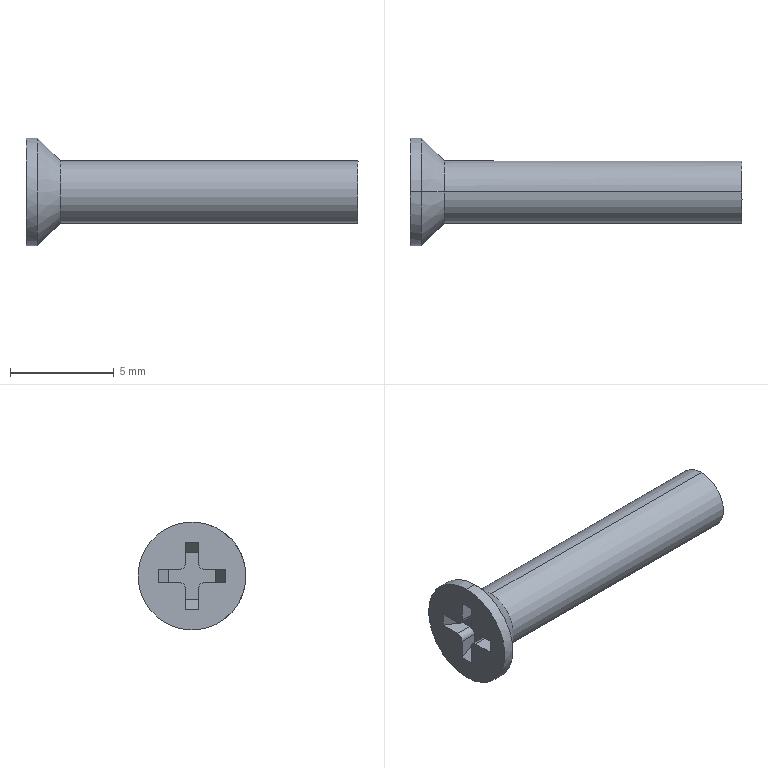Part | STEP file | PN_0006_Default<As Machined> | 1 solid | 25 faces | box 16 x 5.2 x 5.2 mm | volume 125.378 mm3 | plane 15 | cylinder 8 | cone 2 | commonest cylinder face diameters 0.6 x4 3 x2 5.2 x2
STEP:
#1=CARTESIAN_POINT('',(1.65,0.,-1.5));
#2=VERTEX_POINT('',#1);
#3=CARTESIAN_POINT('',(1.65,0.,1.5));
#4=VERTEX_POINT('',#3);
#5=CARTESIAN_POINT('',(1.65,0.,-1.5));
#6=CARTESIAN_POINT('',(1.65,0.4712,-1.5));
#7=CARTESIAN_POINT('',(1.65,0.9425,-1.315));
#8=CARTESIAN_POINT('',(1.65,1.315,-0.9425));
#9=CARTESIAN_POINT('',(1.65,1.685,0.));
#10=CARTESIAN_POINT('',(1.65,1.315,0.9425));
#11=CARTESIAN_POINT('',(1.65,0.9425,1.315));
#12=CARTESIAN_POINT('',(1.65,0.4712,1.5));
#13=CARTESIAN_POINT('',(1.65,0.,1.5));
#14=B_SPLINE_CURVE_WITH_KNOTS('',5,(#5,#6,#7,#8,#9,#10,#11,#12,#13),.UNSPECIFIED.,.F.,.U.,(6,3,6),(-2.356,0.,2.356),.UNSPECIFIED.);
#15=EDGE_CURVE('',#2,#4,#14,.T.);
#16=ORIENTED_EDGE('',*,*,#15,.T.);
#17=CARTESIAN_POINT('',(16.,0.,1.5));
#18=VERTEX_POINT('',#17);
#19=CARTESIAN_POINT('',(4.516,0.,1.5));
#20=DIRECTION('',(1.,0.,0.));
#21=VECTOR('',#20,1.);
#22=LINE('',#19,#21);
#23=EDGE_CURVE('',#4,#18,#22,.T.);
#24=ORIENTED_EDGE('',*,*,#23,.T.);
#25=CARTESIAN_POINT('',(16.,0.,-1.5));
#26=VERTEX_POINT('',#25);
#27=CARTESIAN_POINT('',(16.,0.,0.));
#28=DIRECTION('',(1.,0.,0.));
#29=AXIS2_PLACEMENT_3D('',#27,#28,$);
#30=CIRCLE('',#29,1.5);
#31=EDGE_CURVE('',#26,#18,#30,.T.);
#32=ORIENTED_EDGE('',*,*,#31,.F.);
#33=CARTESIAN_POINT('',(4.516,0.,-1.5));
#34=DIRECTION('',(1.,0.,0.));
#35=VECTOR('',#34,1.);
#36=LINE('',#33,#35);
#37=EDGE_CURVE('',#2,#26,#36,.T.);
#38=ORIENTED_EDGE('',*,*,#37,.F.);
#39=EDGE_LOOP('',(#16,#24,#32,#38));
#40=FACE_OUTER_BOUND('',#39,.T.);
#41=CARTESIAN_POINT('',(4.516,0.,0.));
#42=DIRECTION('',(1.,0.,0.));
#43=DIRECTION('',(0.,0.,-1.));
#44=AXIS2_PLACEMENT_3D('',#41,#42,#43);
#45=CYLINDRICAL_SURFACE('',#44,1.5);
#46=ADVANCED_FACE('',(#40),#45,.T.);
#47=ORIENTED_EDGE('',*,*,#15,.F.);
#48=CARTESIAN_POINT('',(0.55,0.,-2.6));
#49=VERTEX_POINT('',#48);
#50=CARTESIAN_POINT('',(-353550.991,0.,-353554.141));
#51=DIRECTION('',(-0.7071,0.,-0.7071));
#52=VECTOR('',#51,1.);
#53=LINE('',#50,#52);
#54=EDGE_CURVE('',#2,#49,#53,.T.);
#55=ORIENTED_EDGE('',*,*,#54,.T.);
#56=CARTESIAN_POINT('',(0.55,0.,2.6));
#57=VERTEX_POINT('',#56);
#58=CARTESIAN_POINT('',(0.55,0.,0.));
#59=DIRECTION('',(-1.,0.,0.));
#60=AXIS2_PLACEMENT_3D('',#58,#59,$);
#61=CIRCLE('',#60,2.6);
#62=EDGE_CURVE('',#49,#57,#61,.F.);
#63=ORIENTED_EDGE('',*,*,#62,.T.);
#64=CARTESIAN_POINT('',(-353550.991,0.,353554.141));
#65=DIRECTION('',(-0.7071,0.,0.7071));
#66=VECTOR('',#65,1.);
#67=LINE('',#64,#66);
#68=EDGE_CURVE('',#4,#57,#67,.T.);
#69=ORIENTED_EDGE('',*,*,#68,.F.);
#70=EDGE_LOOP('',(#47,#55,#63,#69));
#71=FACE_OUTER_BOUND('',#70,.T.);
#72=CARTESIAN_POINT('',(1.65,0.,0.));
#73=DIRECTION('',(-1.,0.,0.));
#74=DIRECTION('',(0.,0.,1.));
#75=AXIS2_PLACEMENT_3D('',#72,#73,#74);
#76=CONICAL_SURFACE('',#75,1.5,0.7854);
#77=ADVANCED_FACE('',(#71),#76,.T.);
#78=ORIENTED_EDGE('',*,*,#23,.F.);
#79=CARTESIAN_POINT('',(1.65,0.,1.5));
#80=CARTESIAN_POINT('',(1.65,-0.4712,1.5));
#81=CARTESIAN_POINT('',(1.65,-0.9425,1.315));
#82=CARTESIAN_POINT('',(1.65,-1.315,0.9425));
#83=CARTESIAN_POINT('',(1.65,-1.685,0.));
#84=CARTESIAN_POINT('',(1.65,-1.315,-0.9425));
#85=CARTESIAN_POINT('',(1.65,-0.9425,-1.315));
#86=CARTESIAN_POINT('',(1.65,-0.4712,-1.5));
#87=CARTESIAN_POINT('',(1.65,0.,-1.5));
#88=B_SPLINE_CURVE_WITH_KNOTS('',5,(#79,#80,#81,#82,#83,#84,#85,#86,#87),.UNSPECIFIED.,.F.,.U.,(6,3,6),(-2.356,0.,2.356),.UNSPECIFIED.);
#89=EDGE_CURVE('',#4,#2,#88,.T.);
#90=ORIENTED_EDGE('',*,*,#89,.T.);
#91=ORIENTED_EDGE('',*,*,#37,.T.);
#92=CARTESIAN_POINT('',(16.,0.,1.5));
#93=CARTESIAN_POINT('',(16.,-0.4712,1.5));
#94=CARTESIAN_POINT('',(16.,-0.9425,1.315));
#95=CARTESIAN_POINT('',(16.,-1.315,0.9425));
#96=CARTESIAN_POINT('',(16.,-1.685,0.));
#97=CARTESIAN_POINT('',(16.,-1.315,-0.9425));
#98=CARTESIAN_POINT('',(16.,-0.9425,-1.315));
#99=CARTESIAN_POINT('',(16.,-0.4712,-1.5));
#100=CARTESIAN_POINT('',(16.,0.,-1.5));
#101=B_SPLINE_CURVE_WITH_KNOTS('',5,(#92,#93,#94,#95,#96,#97,#98,#99,#100),.UNSPECIFIED.,.F.,.U.,(6,3,6),(-2.356,0.,2.356),.UNSPECIFIED.);
#102=EDGE_CURVE('',#18,#26,#101,.T.);
#103=ORIENTED_EDGE('',*,*,#102,.F.);
#104=EDGE_LOOP('',(#78,#90,#91,#103));
#105=FACE_OUTER_BOUND('',#104,.T.);
#106=CARTESIAN_POINT('',(4.516,0.,0.));
#107=DIRECTION('',(1.,0.,0.));
#108=DIRECTION('',(0.,0.,1.));
#109=AXIS2_PLACEMENT_3D('',#106,#107,#108);
#110=CYLINDRICAL_SURFACE('',#109,1.5);
#111=ADVANCED_FACE('',(#105),#110,.T.);
#112=ORIENTED_EDGE('',*,*,#31,.T.);
#113=ORIENTED_EDGE('',*,*,#102,.T.);
#114=EDGE_LOOP('',(#112,#113));
#115=FACE_OUTER_BOUND('',#114,.T.);
#116=CARTESIAN_POINT('',(16.,1.5,0.));
#117=DIRECTION('',(1.,0.,0.));
#118=DIRECTION('',(0.,0.,-1.));
#119=AXIS2_PLACEMENT_3D('',#116,#117,#118);
#120=PLANE('',#119);
#121=ADVANCED_FACE('',(#115),#120,.T.);
#122=ORIENTED_EDGE('',*,*,#54,.F.);
#123=ORIENTED_EDGE('',*,*,#89,.F.);
#124=ORIENTED_EDGE('',*,*,#68,.T.);
#125=CARTESIAN_POINT('',(0.55,0.,0.));
#126=DIRECTION('',(-1.,0.,0.));
#127=AXIS2_PLACEMENT_3D('',#125,#126,$);
#128=CIRCLE('',#127,2.6);
#129=EDGE_CURVE('',#57,#49,#128,.F.);
#130=ORIENTED_EDGE('',*,*,#129,.T.);
#131=EDGE_LOOP('',(#122,#123,#124,#130));
#132=FACE_OUTER_BOUND('',#131,.T.);
#133=CARTESIAN_POINT('',(1.65,0.,0.));
#134=DIRECTION('',(-1.,0.,0.));
#135=DIRECTION('',(0.,0.,-1.));
#136=AXIS2_PLACEMENT_3D('',#133,#134,#135);
#137=CONICAL_SURFACE('',#136,1.5,0.7854);
#138=ADVANCED_FACE('',(#132),#137,.T.);
#139=CARTESIAN_POINT('',(0.,0.,-2.6));
#140=VERTEX_POINT('',#139);
#141=CARTESIAN_POINT('',(0.,0.,2.6));
#142=VERTEX_POINT('',#141);
#143=CARTESIAN_POINT('',(0.,0.,0.));
#144=DIRECTION('',(1.,0.,0.));
#145=AXIS2_PLACEMENT_3D('',#143,#144,$);
#146=CIRCLE('',#145,2.6);
#147=EDGE_CURVE('',#140,#142,#146,.T.);
#148=ORIENTED_EDGE('',*,*,#147,.T.);
#149=CARTESIAN_POINT('',(4.516,0.,2.6));
#150=DIRECTION('',(1.,0.,0.));
#151=VECTOR('',#150,1.);
#152=LINE('',#149,#151);
#153=EDGE_CURVE('',#142,#57,#152,.T.);
#154=ORIENTED_EDGE('',*,*,#153,.T.);
#155=ORIENTED_EDGE('',*,*,#62,.F.);
#156=CARTESIAN_POINT('',(4.516,0.,-2.6));
#157=DIRECTION('',(1.,0.,0.));
#158=VECTOR('',#157,1.);
#159=LINE('',#156,#158);
#160=EDGE_CURVE('',#140,#49,#159,.T.);
#161=ORIENTED_EDGE('',*,*,#160,.F.);
#162=EDGE_LOOP('',(#148,#154,#155,#161));
#163=FACE_OUTER_BOUND('',#162,.T.);
#164=CARTESIAN_POINT('',(4.516,0.,0.));
#165=DIRECTION('',(1.,0.,0.));
#166=DIRECTION('',(0.,0.,-1.));
#167=AXIS2_PLACEMENT_3D('',#164,#165,#166);
#168=CYLINDRICAL_SURFACE('',#167,2.6);
#169=ADVANCED_FACE('',(#163),#168,.T.);
#170=ORIENTED_EDGE('',*,*,#153,.F.);
#171=CARTESIAN_POINT('',(0.,0.,2.6));
#172=CARTESIAN_POINT('',(0.,-0.8168,2.6));
#173=CARTESIAN_POINT('',(0.,-1.634,2.279));
#174=CARTESIAN_POINT('',(0.,-2.279,1.634));
#175=CARTESIAN_POINT('',(0.,-2.921,0.));
#176=CARTESIAN_POINT('',(0.,-2.279,-1.634));
#177=CARTESIAN_POINT('',(0.,-1.634,-2.279));
#178=CARTESIAN_POINT('',(0.,-0.8168,-2.6));
#179=CARTESIAN_POINT('',(0.,0.,-2.6));
#180=B_SPLINE_CURVE_WITH_KNOTS('',5,(#171,#172,#173,#174,#175,#176,#177,#178,#179),.UNSPECIFIED.,.F.,.U.,(6,3,6),(-4.084,0.,4.084),.UNSPECIFIED.);
#181=EDGE_CURVE('',#142,#140,#180,.T.);
#182=ORIENTED_EDGE('',*,*,#181,.T.);
#183=ORIENTED_EDGE('',*,*,#160,.T.);
#184=ORIENTED_EDGE('',*,*,#129,.F.);
#185=EDGE_LOOP('',(#170,#182,#183,#184));
#186=FACE_OUTER_BOUND('',#185,.T.);
#187=CARTESIAN_POINT('',(4.516,0.,0.));
#188=DIRECTION('',(1.,0.,0.));
#189=DIRECTION('',(0.,0.,1.));
#190=AXIS2_PLACEMENT_3D('',#187,#188,#189);
#191=CYLINDRICAL_SURFACE('',#190,2.6);
#192=ADVANCED_FACE('',(#186),#191,.T.);
#193=ORIENTED_EDGE('',*,*,#147,.F.);
#194=ORIENTED_EDGE('',*,*,#181,.F.);
#195=EDGE_LOOP('',(#193,#194));
#196=FACE_OUTER_BOUND('',#195,.T.);
#197=CARTESIAN_POINT('',(0.,-1.6,-0.32));
#198=VERTEX_POINT('',#197);
#199=CARTESIAN_POINT('',(0.,-0.62,-0.32));
#200=VERTEX_POINT('',#199);
#201=CARTESIAN_POINT('',(0.,-1.11,-0.32));
#202=DIRECTION('',(0.,1.,0.));
#203=VECTOR('',#202,1.);
#204=LINE('',#201,#203);
#205=EDGE_CURVE('',#198,#200,#204,.T.);
#206=ORIENTED_EDGE('',*,*,#205,.T.);
#207=CARTESIAN_POINT('',(0.,-0.32,-0.62));
#208=VERTEX_POINT('',#207);
#209=CARTESIAN_POINT('',(0.,-0.62,-0.62));
#210=DIRECTION('',(-1.,0.,0.));
#211=AXIS2_PLACEMENT_3D('',#209,#210,$);
#212=CIRCLE('',#211,0.3);
#213=EDGE_CURVE('',#200,#208,#212,.T.);
#214=ORIENTED_EDGE('',*,*,#213,.T.);
#215=CARTESIAN_POINT('',(0.,-0.32,-1.6));
#216=VERTEX_POINT('',#215);
#217=CARTESIAN_POINT('',(0.,-0.32,-1.11));
#218=DIRECTION('',(0.,0.,-1.));
#219=VECTOR('',#218,1.);
#220=LINE('',#217,#219);
#221=EDGE_CURVE('',#208,#216,#220,.T.);
#222=ORIENTED_EDGE('',*,*,#221,.T.);
#223=CARTESIAN_POINT('',(0.,0.32,-1.6));
#224=VERTEX_POINT('',#223);
#225=CARTESIAN_POINT('',(0.,0.,-1.6));
#226=DIRECTION('',(0.,1.,0.));
#227=VECTOR('',#226,1.);
#228=LINE('',#225,#227);
#229=EDGE_CURVE('',#216,#224,#228,.T.);
#230=ORIENTED_EDGE('',*,*,#229,.T.);
#231=CARTESIAN_POINT('',(0.,0.32,-0.62));
#232=VERTEX_POINT('',#231);
#233=CARTESIAN_POINT('',(0.,0.32,-1.11));
#234=DIRECTION('',(0.,0.,1.));
#235=VECTOR('',#234,1.);
#236=LINE('',#233,#235);
#237=EDGE_CURVE('',#224,#232,#236,.T.);
#238=ORIENTED_EDGE('',*,*,#237,.T.);
#239=CARTESIAN_POINT('',(0.,0.62,-0.32));
#240=VERTEX_POINT('',#239);
#241=CARTESIAN_POINT('',(0.,0.62,-0.62));
#242=DIRECTION('',(-1.,0.,0.));
#243=AXIS2_PLACEMENT_3D('',#241,#242,$);
#244=CIRCLE('',#243,0.3);
#245=EDGE_CURVE('',#232,#240,#244,.T.);
#246=ORIENTED_EDGE('',*,*,#245,.T.);
#247=CARTESIAN_POINT('',(0.,1.6,-0.32));
#248=VERTEX_POINT('',#247);
#249=CARTESIAN_POINT('',(0.,1.11,-0.32));
#250=DIRECTION('',(0.,1.,0.));
#251=VECTOR('',#250,1.);
#252=LINE('',#249,#251);
#253=EDGE_CURVE('',#240,#248,#252,.T.);
#254=ORIENTED_EDGE('',*,*,#253,.T.);
#255=CARTESIAN_POINT('',(0.,1.6,0.32));
#256=VERTEX_POINT('',#255);
#257=CARTESIAN_POINT('',(0.,1.6,0.));
#258=DIRECTION('',(0.,0.,1.));
#259=VECTOR('',#258,1.);
#260=LINE('',#257,#259);
#261=EDGE_CURVE('',#248,#256,#260,.T.);
#262=ORIENTED_EDGE('',*,*,#261,.T.);
#263=CARTESIAN_POINT('',(0.,0.62,0.32));
#264=VERTEX_POINT('',#263);
#265=CARTESIAN_POINT('',(0.,1.11,0.32));
#266=DIRECTION('',(0.,-1.,0.));
#267=VECTOR('',#266,1.);
#268=LINE('',#265,#267);
#269=EDGE_CURVE('',#256,#264,#268,.T.);
#270=ORIENTED_EDGE('',*,*,#269,.T.);
#271=CARTESIAN_POINT('',(0.,0.32,0.62));
#272=VERTEX_POINT('',#271);
#273=CARTESIAN_POINT('',(0.,0.62,0.62));
#274=DIRECTION('',(-1.,0.,0.));
#275=AXIS2_PLACEMENT_3D('',#273,#274,$);
#276=CIRCLE('',#275,0.3);
#277=EDGE_CURVE('',#264,#272,#276,.T.);
#278=ORIENTED_EDGE('',*,*,#277,.T.);
#279=CARTESIAN_POINT('',(0.,0.32,1.6));
#280=VERTEX_POINT('',#279);
#281=CARTESIAN_POINT('',(0.,0.32,1.11));
#282=DIRECTION('',(0.,0.,1.));
#283=VECTOR('',#282,1.);
#284=LINE('',#281,#283);
#285=EDGE_CURVE('',#272,#280,#284,.T.);
#286=ORIENTED_EDGE('',*,*,#285,.T.);
#287=CARTESIAN_POINT('',(0.,-0.32,1.6));
#288=VERTEX_POINT('',#287);
#289=CARTESIAN_POINT('',(0.,0.,1.6));
#290=DIRECTION('',(0.,-1.,0.));
#291=VECTOR('',#290,1.);
#292=LINE('',#289,#291);
#293=EDGE_CURVE('',#280,#288,#292,.T.);
#294=ORIENTED_EDGE('',*,*,#293,.T.);
#295=CARTESIAN_POINT('',(0.,-0.32,0.62));
#296=VERTEX_POINT('',#295);
#297=CARTESIAN_POINT('',(0.,-0.32,1.11));
#298=DIRECTION('',(0.,0.,-1.));
#299=VECTOR('',#298,1.);
#300=LINE('',#297,#299);
#301=EDGE_CURVE('',#288,#296,#300,.T.);
#302=ORIENTED_EDGE('',*,*,#301,.T.);
#303=CARTESIAN_POINT('',(0.,-0.62,0.32));
#304=VERTEX_POINT('',#303);
#305=CARTESIAN_POINT('',(0.,-0.62,0.62));
#306=DIRECTION('',(-1.,0.,0.));
#307=AXIS2_PLACEMENT_3D('',#305,#306,$);
#308=CIRCLE('',#307,0.3);
#309=EDGE_CURVE('',#296,#304,#308,.T.);
#310=ORIENTED_EDGE('',*,*,#309,.T.);
#311=CARTESIAN_POINT('',(0.,-1.6,0.32));
#312=VERTEX_POINT('',#311);
#313=CARTESIAN_POINT('',(0.,-1.11,0.32));
#314=DIRECTION('',(0.,-1.,0.));
#315=VECTOR('',#314,1.);
#316=LINE('',#313,#315);
#317=EDGE_CURVE('',#304,#312,#316,.T.);
#318=ORIENTED_EDGE('',*,*,#317,.T.);
#319=CARTESIAN_POINT('',(0.,-1.6,0.));
#320=DIRECTION('',(0.,0.,-1.));
#321=VECTOR('',#320,1.);
#322=LINE('',#319,#321);
#323=EDGE_CURVE('',#312,#198,#322,.T.);
#324=ORIENTED_EDGE('',*,*,#323,.T.);
#325=EDGE_LOOP('',(#206,#214,#222,#230,#238,#246,#254,#262,#270,#278,#286,#294,#302,#310,#318,#324));
#326=FACE_BOUND('',#325,.T.);
#327=CARTESIAN_POINT('',(0.,2.6,0.));
#328=DIRECTION('',(-1.,0.,0.));
#329=DIRECTION('',(0.,0.,1.));
#330=AXIS2_PLACEMENT_3D('',#327,#328,#329);
#331=PLANE('',#330);
#332=ADVANCED_FACE('',(#196,#326),#331,.T.);
#333=CARTESIAN_POINT('',(0.825,-1.124,-0.32));
#334=VERTEX_POINT('',#333);
#335=CARTESIAN_POINT('',(0.825,-0.62,-0.32));
#336=VERTEX_POINT('',#335);
#337=CARTESIAN_POINT('',(0.825,-0.8718,-0.32));
#338=DIRECTION('',(0.,1.,0.));
#339=VECTOR('',#338,1.);
#340=LINE('',#337,#339);
#341=EDGE_CURVE('',#334,#336,#340,.T.);
#342=ORIENTED_EDGE('',*,*,#341,.T.);
#343=CARTESIAN_POINT('',(0.4125,-0.62,-0.32));
#344=DIRECTION('',(-1.,0.,0.));
#345=VECTOR('',#344,1.);
#346=LINE('',#343,#345);
#347=EDGE_CURVE('',#336,#200,#346,.T.);
#348=ORIENTED_EDGE('',*,*,#347,.T.);
#349=ORIENTED_EDGE('',*,*,#205,.F.);
#350=CARTESIAN_POINT('',(0.4125,-1.362,-0.32));
#351=DIRECTION('',(-0.866,-0.5,0.));
#352=VECTOR('',#351,1.);
#353=LINE('',#350,#352);
#354=EDGE_CURVE('',#334,#198,#353,.T.);
#355=ORIENTED_EDGE('',*,*,#354,.F.);
#356=EDGE_LOOP('',(#342,#348,#349,#355));
#357=FACE_OUTER_BOUND('',#356,.T.);
#358=CARTESIAN_POINT('',(0.825,-0.32,-0.32));
#359=DIRECTION('',(0.,0.,1.));
#360=DIRECTION('',(1.,0.,0.));
#361=AXIS2_PLACEMENT_3D('',#358,#359,#360);
#362=PLANE('',#361);
#363=ADVANCED_FACE('',(#357),#362,.T.);
#364=CARTESIAN_POINT('',(0.825,-0.32,-0.62));
#365=VERTEX_POINT('',#364);
#366=CARTESIAN_POINT('',(0.825,-0.62,-0.62));
#367=DIRECTION('',(-1.,0.,0.));
#368=AXIS2_PLACEMENT_3D('',#366,#367,$);
#369=CIRCLE('',#368,0.3);
#370=EDGE_CURVE('',#365,#336,#369,.F.);
#371=ORIENTED_EDGE('',*,*,#370,.F.);
#372=CARTESIAN_POINT('',(0.825,-0.32,-0.62));
#373=DIRECTION('',(-1.,0.,0.));
#374=VECTOR('',#373,1.);
#375=LINE('',#372,#374);
#376=EDGE_CURVE('',#208,#365,#375,.F.);
#377=ORIENTED_EDGE('',*,*,#376,.F.);
#378=ORIENTED_EDGE('',*,*,#213,.F.);
#379=ORIENTED_EDGE('',*,*,#347,.F.);
#380=EDGE_LOOP('',(#371,#377,#378,#379));
#381=FACE_OUTER_BOUND('',#380,.T.);
#382=CARTESIAN_POINT('',(0.825,-0.62,-0.62));
#383=DIRECTION('',(-1.,0.,0.));
#384=DIRECTION('',(0.,0.,1.));
#385=AXIS2_PLACEMENT_3D('',#382,#383,#384);
#386=CYLINDRICAL_SURFACE('',#385,0.3);
#387=ADVANCED_FACE('',(#381),#386,.T.);
#388=ORIENTED_EDGE('',*,*,#221,.F.);
#389=ORIENTED_EDGE('',*,*,#376,.T.);
#390=CARTESIAN_POINT('',(0.825,-0.32,-1.124));
#391=VERTEX_POINT('',#390);
#392=CARTESIAN_POINT('',(0.825,-0.32,-0.8718));
#393=DIRECTION('',(0.,0.,-1.));
#394=VECTOR('',#393,1.);
#395=LINE('',#392,#394);
#396=EDGE_CURVE('',#365,#391,#395,.T.);
#397=ORIENTED_EDGE('',*,*,#396,.T.);
#398=CARTESIAN_POINT('',(0.4125,-0.32,-1.362));
#399=DIRECTION('',(-0.866,0.,-0.5));
#400=VECTOR('',#399,1.);
#401=LINE('',#398,#400);
#402=EDGE_CURVE('',#391,#216,#401,.T.);
#403=ORIENTED_EDGE('',*,*,#402,.T.);
#404=EDGE_LOOP('',(#388,#389,#397,#403));
#405=FACE_OUTER_BOUND('',#404,.T.);
#406=CARTESIAN_POINT('',(0.825,-0.32,-0.32));
#407=DIRECTION('',(0.,1.,0.));
#408=DIRECTION('',(0.,0.,1.));
#409=AXIS2_PLACEMENT_3D('',#406,#407,#408);
#410=PLANE('',#409);
#411=ADVANCED_FACE('',(#405),#410,.T.);
#412=ORIENTED_EDGE('',*,*,#229,.F.);
#413=ORIENTED_EDGE('',*,*,#402,.F.);
#414=CARTESIAN_POINT('',(0.825,0.32,-1.124));
#415=VERTEX_POINT('',#414);
#416=CARTESIAN_POINT('',(0.825,0.,-1.124));
#417=DIRECTION('',(0.,1.,0.));
#418=VECTOR('',#417,1.);
#419=LINE('',#416,#418);
#420=EDGE_CURVE('',#391,#415,#419,.T.);
#421=ORIENTED_EDGE('',*,*,#420,.T.);
#422=CARTESIAN_POINT('',(0.4125,0.32,-1.362));
#423=DIRECTION('',(-0.866,0.,-0.5));
#424=VECTOR('',#423,1.);
#425=LINE('',#422,#424);
#426=EDGE_CURVE('',#415,#224,#425,.T.);
#427=ORIENTED_EDGE('',*,*,#426,.T.);
#428=EDGE_LOOP('',(#412,#413,#421,#427));
#429=FACE_OUTER_BOUND('',#428,.T.);
#430=CARTESIAN_POINT('',(0.,0.32,-1.6));
#431=DIRECTION('',(-0.5,0.,0.866));
#432=DIRECTION('',(0.866,0.,0.5));
#433=AXIS2_PLACEMENT_3D('',#430,#431,#432);
#434=PLANE('',#433);
#435=ADVANCED_FACE('',(#429),#434,.T.);
#436=CARTESIAN_POINT('',(0.825,0.32,-0.62));
#437=VERTEX_POINT('',#436);
#438=CARTESIAN_POINT('',(0.825,0.32,-0.8718));
#439=DIRECTION('',(0.,0.,1.));
#440=VECTOR('',#439,1.);
#441=LINE('',#438,#440);
#442=EDGE_CURVE('',#415,#437,#441,.T.);
#443=ORIENTED_EDGE('',*,*,#442,.T.);
#444=CARTESIAN_POINT('',(0.4125,0.32,-0.62));
#445=DIRECTION('',(-1.,0.,0.));
#446=VECTOR('',#445,1.);
#447=LINE('',#444,#446);
#448=EDGE_CURVE('',#437,#232,#447,.T.);
#449=ORIENTED_EDGE('',*,*,#448,.T.);
#450=ORIENTED_EDGE('',*,*,#237,.F.);
#451=ORIENTED_EDGE('',*,*,#426,.F.);
#452=EDGE_LOOP('',(#443,#449,#450,#451));
#453=FACE_OUTER_BOUND('',#452,.T.);
#454=CARTESIAN_POINT('',(0.825,0.32,-0.32));
#455=DIRECTION('',(0.,-1.,0.));
#456=DIRECTION('',(0.,0.,-1.));
#457=AXIS2_PLACEMENT_3D('',#454,#455,#456);
#458=PLANE('',#457);
#459=ADVANCED_FACE('',(#453),#458,.T.);
#460=CARTESIAN_POINT('',(0.825,0.62,-0.32));
#461=VERTEX_POINT('',#460);
#462=CARTESIAN_POINT('',(0.825,0.62,-0.62));
#463=DIRECTION('',(-1.,0.,0.));
#464=AXIS2_PLACEMENT_3D('',#462,#463,$);
#465=CIRCLE('',#464,0.3);
#466=EDGE_CURVE('',#461,#437,#465,.F.);
#467=ORIENTED_EDGE('',*,*,#466,.F.);
#468=CARTESIAN_POINT('',(0.825,0.62,-0.32));
#469=DIRECTION('',(-1.,0.,0.));
#470=VECTOR('',#469,1.);
#471=LINE('',#468,#470);
#472=EDGE_CURVE('',#240,#461,#471,.F.);
#473=ORIENTED_EDGE('',*,*,#472,.F.);
#474=ORIENTED_EDGE('',*,*,#245,.F.);
#475=ORIENTED_EDGE('',*,*,#448,.F.);
#476=EDGE_LOOP('',(#467,#473,#474,#475));
#477=FACE_OUTER_BOUND('',#476,.T.);
#478=CARTESIAN_POINT('',(0.825,0.62,-0.62));
#479=DIRECTION('',(-1.,0.,0.));
#480=DIRECTION('',(0.,0.,-1.));
#481=AXIS2_PLACEMENT_3D('',#478,#479,#480);
#482=CYLINDRICAL_SURFACE('',#481,0.3);
#483=ADVANCED_FACE('',(#477),#482,.T.);
#484=ORIENTED_EDGE('',*,*,#253,.F.);
#485=ORIENTED_EDGE('',*,*,#472,.T.);
#486=CARTESIAN_POINT('',(0.825,1.124,-0.32));
#487=VERTEX_POINT('',#486);
#488=CARTESIAN_POINT('',(0.825,0.8718,-0.32));
#489=DIRECTION('',(0.,1.,0.));
#490=VECTOR('',#489,1.);
#491=LINE('',#488,#490);
#492=EDGE_CURVE('',#461,#487,#491,.T.);
#493=ORIENTED_EDGE('',*,*,#492,.T.);
#494=CARTESIAN_POINT('',(0.4125,1.362,-0.32));
#495=DIRECTION('',(-0.866,0.5,0.));
#496=VECTOR('',#495,1.);
#497=LINE('',#494,#496);
#498=EDGE_CURVE('',#487,#248,#497,.T.);
#499=ORIENTED_EDGE('',*,*,#498,.T.);
#500=EDGE_LOOP('',(#484,#485,#493,#499));
#501=FACE_OUTER_BOUND('',#500,.T.);
#502=CARTESIAN_POINT('',(0.825,0.32,-0.32));
#503=DIRECTION('',(0.,0.,1.));
#504=DIRECTION('',(1.,0.,0.));
#505=AXIS2_PLACEMENT_3D('',#502,#503,#504);
#506=PLANE('',#505);
#507=ADVANCED_FACE('',(#501),#506,.T.);
#508=ORIENTED_EDGE('',*,*,#261,.F.);
#509=ORIENTED_EDGE('',*,*,#498,.F.);
#510=CARTESIAN_POINT('',(0.825,1.124,0.32));
#511=VERTEX_POINT('',#510);
#512=CARTESIAN_POINT('',(0.825,1.124,0.));
#513=DIRECTION('',(0.,0.,1.));
#514=VECTOR('',#513,1.);
#515=LINE('',#512,#514);
#516=EDGE_CURVE('',#487,#511,#515,.T.);
#517=ORIENTED_EDGE('',*,*,#516,.T.);
#518=CARTESIAN_POINT('',(0.4125,1.362,0.32));
#519=DIRECTION('',(-0.866,0.5,0.));
#520=VECTOR('',#519,1.);
#521=LINE('',#518,#520);
#522=EDGE_CURVE('',#511,#256,#521,.T.);
#523=ORIENTED_EDGE('',*,*,#522,.T.);
#524=EDGE_LOOP('',(#508,#509,#517,#523));
#525=FACE_OUTER_BOUND('',#524,.T.);
#526=CARTESIAN_POINT('',(0.,1.6,-0.32));
#527=DIRECTION('',(-0.5,-0.866,0.));
#528=DIRECTION('',(0.866,-0.5,0.));
#529=AXIS2_PLACEMENT_3D('',#526,#527,#528);
#530=PLANE('',#529);
#531=ADVANCED_FACE('',(#525),#530,.T.);
#532=CARTESIAN_POINT('',(0.825,0.62,0.32));
#533=VERTEX_POINT('',#532);
#534=CARTESIAN_POINT('',(0.825,0.8718,0.32));
#535=DIRECTION('',(0.,-1.,0.));
#536=VECTOR('',#535,1.);
#537=LINE('',#534,#536);
#538=EDGE_CURVE('',#511,#533,#537,.T.);
#539=ORIENTED_EDGE('',*,*,#538,.T.);
#540=CARTESIAN_POINT('',(0.4125,0.62,0.32));
#541=DIRECTION('',(-1.,0.,0.));
#542=VECTOR('',#541,1.);
#543=LINE('',#540,#542);
#544=EDGE_CURVE('',#533,#264,#543,.T.);
#545=ORIENTED_EDGE('',*,*,#544,.T.);
#546=ORIENTED_EDGE('',*,*,#269,.F.);
#547=ORIENTED_EDGE('',*,*,#522,.F.);
#548=EDGE_LOOP('',(#539,#545,#546,#547));
#549=FACE_OUTER_BOUND('',#548,.T.);
#550=CARTESIAN_POINT('',(0.825,0.32,0.32));
#551=DIRECTION('',(0.,0.,-1.));
#552=DIRECTION('',(0.,1.,0.));
#553=AXIS2_PLACEMENT_3D('',#550,#551,#552);
#554=PLANE('',#553);
#555=ADVANCED_FACE('',(#549),#554,.T.);
#556=CARTESIAN_POINT('',(0.825,0.32,0.62));
#557=VERTEX_POINT('',#556);
#558=CARTESIAN_POINT('',(0.825,0.62,0.62));
#559=DIRECTION('',(-1.,0.,0.));
#560=AXIS2_PLACEMENT_3D('',#558,#559,$);
#561=CIRCLE('',#560,0.3);
#562=EDGE_CURVE('',#557,#533,#561,.F.);
#563=ORIENTED_EDGE('',*,*,#562,.F.);
#564=CARTESIAN_POINT('',(0.825,0.32,0.62));
#565=DIRECTION('',(-1.,0.,0.));
#566=VECTOR('',#565,1.);
#567=LINE('',#564,#566);
#568=EDGE_CURVE('',#272,#557,#567,.F.);
#569=ORIENTED_EDGE('',*,*,#568,.F.);
#570=ORIENTED_EDGE('',*,*,#277,.F.);
#571=ORIENTED_EDGE('',*,*,#544,.F.);
#572=EDGE_LOOP('',(#563,#569,#570,#571));
#573=FACE_OUTER_BOUND('',#572,.T.);
#574=CARTESIAN_POINT('',(0.825,0.62,0.62));
#575=DIRECTION('',(-1.,0.,0.));
#576=DIRECTION('',(0.,0.,-1.));
#577=AXIS2_PLACEMENT_3D('',#574,#575,#576);
#578=CYLINDRICAL_SURFACE('',#577,0.3);
#579=ADVANCED_FACE('',(#573),#578,.T.);
#580=ORIENTED_EDGE('',*,*,#285,.F.);
#581=ORIENTED_EDGE('',*,*,#568,.T.);
#582=CARTESIAN_POINT('',(0.825,0.32,1.124));
#583=VERTEX_POINT('',#582);
#584=CARTESIAN_POINT('',(0.825,0.32,0.8718));
#585=DIRECTION('',(0.,0.,1.));
#586=VECTOR('',#585,1.);
#587=LINE('',#584,#586);
#588=EDGE_CURVE('',#557,#583,#587,.T.);
#589=ORIENTED_EDGE('',*,*,#588,.T.);
#590=CARTESIAN_POINT('',(0.4125,0.32,1.362));
#591=DIRECTION('',(-0.866,0.,0.5));
#592=VECTOR('',#591,1.);
#593=LINE('',#590,#592);
#594=EDGE_CURVE('',#583,#280,#593,.T.);
#595=ORIENTED_EDGE('',*,*,#594,.T.);
#596=EDGE_LOOP('',(#580,#581,#589,#595));
#597=FACE_OUTER_BOUND('',#596,.T.);
#598=CARTESIAN_POINT('',(0.825,0.32,0.32));
#599=DIRECTION('',(0.,-1.,0.));
#600=DIRECTION('',(0.,0.,-1.));
#601=AXIS2_PLACEMENT_3D('',#598,#599,#600);
#602=PLANE('',#601);
#603=ADVANCED_FACE('',(#597),#602,.T.);
#604=ORIENTED_EDGE('',*,*,#293,.F.);
#605=ORIENTED_EDGE('',*,*,#594,.F.);
#606=CARTESIAN_POINT('',(0.825,-0.32,1.124));
#607=VERTEX_POINT('',#606);
#608=CARTESIAN_POINT('',(0.825,0.,1.124));
#609=DIRECTION('',(0.,-1.,0.));
#610=VECTOR('',#609,1.);
#611=LINE('',#608,#610);
#612=EDGE_CURVE('',#583,#607,#611,.T.);
#613=ORIENTED_EDGE('',*,*,#612,.T.);
#614=CARTESIAN_POINT('',(0.4125,-0.32,1.362));
#615=DIRECTION('',(-0.866,0.,0.5));
#616=VECTOR('',#615,1.);
#617=LINE('',#614,#616);
#618=EDGE_CURVE('',#607,#288,#617,.T.);
#619=ORIENTED_EDGE('',*,*,#618,.T.);
#620=EDGE_LOOP('',(#604,#605,#613,#619));
#621=FACE_OUTER_BOUND('',#620,.T.);
#622=CARTESIAN_POINT('',(0.,0.32,1.6));
#623=DIRECTION('',(-0.5,0.,-0.866));
#624=DIRECTION('',(-0.866,0.,0.5));
#625=AXIS2_PLACEMENT_3D('',#622,#623,#624);
#626=PLANE('',#625);
#627=ADVANCED_FACE('',(#621),#626,.T.);
#628=CARTESIAN_POINT('',(0.825,-0.32,0.62));
#629=VERTEX_POINT('',#628);
#630=CARTESIAN_POINT('',(0.825,-0.32,0.8718));
#631=DIRECTION('',(0.,0.,-1.));
#632=VECTOR('',#631,1.);
#633=LINE('',#630,#632);
#634=EDGE_CURVE('',#607,#629,#633,.T.);
#635=ORIENTED_EDGE('',*,*,#634,.T.);
#636=CARTESIAN_POINT('',(0.4125,-0.32,0.62));
#637=DIRECTION('',(-1.,0.,0.));
#638=VECTOR('',#637,1.);
#639=LINE('',#636,#638);
#640=EDGE_CURVE('',#629,#296,#639,.T.);
#641=ORIENTED_EDGE('',*,*,#640,.T.);
#642=ORIENTED_EDGE('',*,*,#301,.F.);
#643=ORIENTED_EDGE('',*,*,#618,.F.);
#644=EDGE_LOOP('',(#635,#641,#642,#643));
#645=FACE_OUTER_BOUND('',#644,.T.);
#646=CARTESIAN_POINT('',(0.825,-0.32,0.32));
#647=DIRECTION('',(0.,1.,0.));
#648=DIRECTION('',(0.,0.,1.));
#649=AXIS2_PLACEMENT_3D('',#646,#647,#648);
#650=PLANE('',#649);
#651=ADVANCED_FACE('',(#645),#650,.T.);
#652=CARTESIAN_POINT('',(0.825,-0.62,0.32));
#653=VERTEX_POINT('',#652);
#654=CARTESIAN_POINT('',(0.825,-0.62,0.62));
#655=DIRECTION('',(-1.,0.,0.));
#656=AXIS2_PLACEMENT_3D('',#654,#655,$);
#657=CIRCLE('',#656,0.3);
#658=EDGE_CURVE('',#653,#629,#657,.F.);
#659=ORIENTED_EDGE('',*,*,#658,.F.);
#660=CARTESIAN_POINT('',(0.825,-0.62,0.32));
#661=DIRECTION('',(-1.,0.,0.));
#662=VECTOR('',#661,1.);
#663=LINE('',#660,#662);
#664=EDGE_CURVE('',#304,#653,#663,.F.);
#665=ORIENTED_EDGE('',*,*,#664,.F.);
#666=ORIENTED_EDGE('',*,*,#309,.F.);
#667=ORIENTED_EDGE('',*,*,#640,.F.);
#668=EDGE_LOOP('',(#659,#665,#666,#667));
#669=FACE_OUTER_BOUND('',#668,.T.);
#670=CARTESIAN_POINT('',(0.825,-0.62,0.62));
#671=DIRECTION('',(-1.,0.,0.));
#672=DIRECTION('',(0.,0.,1.));
#673=AXIS2_PLACEMENT_3D('',#670,#671,#672);
#674=CYLINDRICAL_SURFACE('',#673,0.3);
#675=ADVANCED_FACE('',(#669),#674,.T.);
#676=ORIENTED_EDGE('',*,*,#317,.F.);
#677=ORIENTED_EDGE('',*,*,#664,.T.);
#678=CARTESIAN_POINT('',(0.825,-1.124,0.32));
#679=VERTEX_POINT('',#678);
#680=CARTESIAN_POINT('',(0.825,-0.8718,0.32));
#681=DIRECTION('',(0.,-1.,0.));
#682=VECTOR('',#681,1.);
#683=LINE('',#680,#682);
#684=EDGE_CURVE('',#653,#679,#683,.T.);
#685=ORIENTED_EDGE('',*,*,#684,.T.);
#686=CARTESIAN_POINT('',(0.4125,-1.362,0.32));
#687=DIRECTION('',(-0.866,-0.5,0.));
#688=VECTOR('',#687,1.);
#689=LINE('',#686,#688);
#690=EDGE_CURVE('',#679,#312,#689,.T.);
#691=ORIENTED_EDGE('',*,*,#690,.T.);
#692=EDGE_LOOP('',(#676,#677,#685,#691));
#693=FACE_OUTER_BOUND('',#692,.T.);
#694=CARTESIAN_POINT('',(0.825,-0.32,0.32));
#695=DIRECTION('',(0.,0.,-1.));
#696=DIRECTION('',(0.,1.,0.));
#697=AXIS2_PLACEMENT_3D('',#694,#695,#696);
#698=PLANE('',#697);
#699=ADVANCED_FACE('',(#693),#698,.T.);
#700=ORIENTED_EDGE('',*,*,#323,.F.);
#701=ORIENTED_EDGE('',*,*,#690,.F.);
#702=CARTESIAN_POINT('',(0.825,-1.124,0.));
#703=DIRECTION('',(0.,0.,-1.));
#704=VECTOR('',#703,1.);
#705=LINE('',#702,#704);
#706=EDGE_CURVE('',#679,#334,#705,.T.);
#707=ORIENTED_EDGE('',*,*,#706,.T.);
#708=ORIENTED_EDGE('',*,*,#354,.T.);
#709=EDGE_LOOP('',(#700,#701,#707,#708));
#710=FACE_OUTER_BOUND('',#709,.T.);
#711=CARTESIAN_POINT('',(0.,-1.6,-0.32));
#712=DIRECTION('',(-0.5,0.866,0.));
#713=DIRECTION('',(-0.866,-0.5,0.));
#714=AXIS2_PLACEMENT_3D('',#711,#712,#713);
#715=PLANE('',#714);
#716=ADVANCED_FACE('',(#710),#715,.T.);
#717=ORIENTED_EDGE('',*,*,#588,.F.);
#718=ORIENTED_EDGE('',*,*,#562,.T.);
#719=ORIENTED_EDGE('',*,*,#538,.F.);
#720=ORIENTED_EDGE('',*,*,#516,.F.);
#721=ORIENTED_EDGE('',*,*,#492,.F.);
#722=ORIENTED_EDGE('',*,*,#466,.T.);
#723=ORIENTED_EDGE('',*,*,#442,.F.);
#724=ORIENTED_EDGE('',*,*,#420,.F.);
#725=ORIENTED_EDGE('',*,*,#396,.F.);
#726=ORIENTED_EDGE('',*,*,#370,.T.);
#727=ORIENTED_EDGE('',*,*,#341,.F.);
#728=ORIENTED_EDGE('',*,*,#706,.F.);
#729=ORIENTED_EDGE('',*,*,#684,.F.);
#730=ORIENTED_EDGE('',*,*,#658,.T.);
#731=ORIENTED_EDGE('',*,*,#634,.F.);
#732=ORIENTED_EDGE('',*,*,#612,.F.);
#733=EDGE_LOOP('',(#717,#718,#719,#720,#721,#722,#723,#724,#725,#726,#727,#728,#729,#730,#731,#732));
#734=FACE_OUTER_BOUND('',#733,.T.);
#735=CARTESIAN_POINT('',(0.825,0.32,0.32));
#736=DIRECTION('',(1.,0.,0.));
#737=DIRECTION('',(0.,0.,-1.));
#738=AXIS2_PLACEMENT_3D('',#735,#736,#737);
#739=PLANE('',#738);
#740=ADVANCED_FACE('',(#734),#739,.F.);
#741=CLOSED_SHELL('',(#46,#77,#111,#121,#138,#169,#192,#332,#363,#387,#411,#435,#459,#483,#507,#531,#555,#579,#603,#627,#651,#675,#699,#716,#740));
#742=MANIFOLD_SOLID_BREP('',#741);
#743=(LENGTH_UNIT()NAMED_UNIT(*)SI_UNIT(.MILLI.,.METRE.));
#744=UNCERTAINTY_MEASURE_WITH_UNIT(LENGTH_MEASURE(0.005),#743,'','');
#745=(NAMED_UNIT(*)PLANE_ANGLE_UNIT()SI_UNIT($,.RADIAN.));
#746=(NAMED_UNIT(*)SI_UNIT($,.STERADIAN.)SOLID_ANGLE_UNIT());
#747=(GEOMETRIC_REPRESENTATION_CONTEXT(3)GLOBAL_UNCERTAINTY_ASSIGNED_CONTEXT((#744))GLOBAL_UNIT_ASSIGNED_CONTEXT((#743,#745,#746))REPRESENTATION_CONTEXT('',''));
#748=ADVANCED_BREP_SHAPE_REPRESENTATION('',(#742),#747);